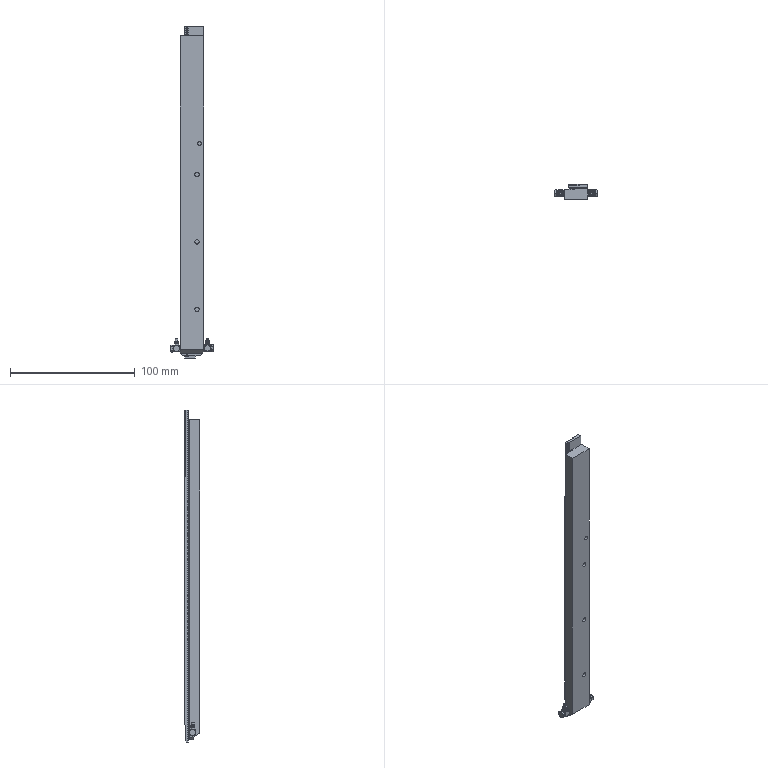Part | SolidWorks | features ReferencePattern 2, LocalLPattern 1 | 7 solids | 588 faces | box 33.8 x 12.35 x 265.95 mm | volume 52246 mm3 | plane 269 | spline 151 | cylinder 120 | cone 48 | commonest cylinder face diameters 0.2 x18 0.4 x18 2.5 x14 5 x8 2 x7 3 x7